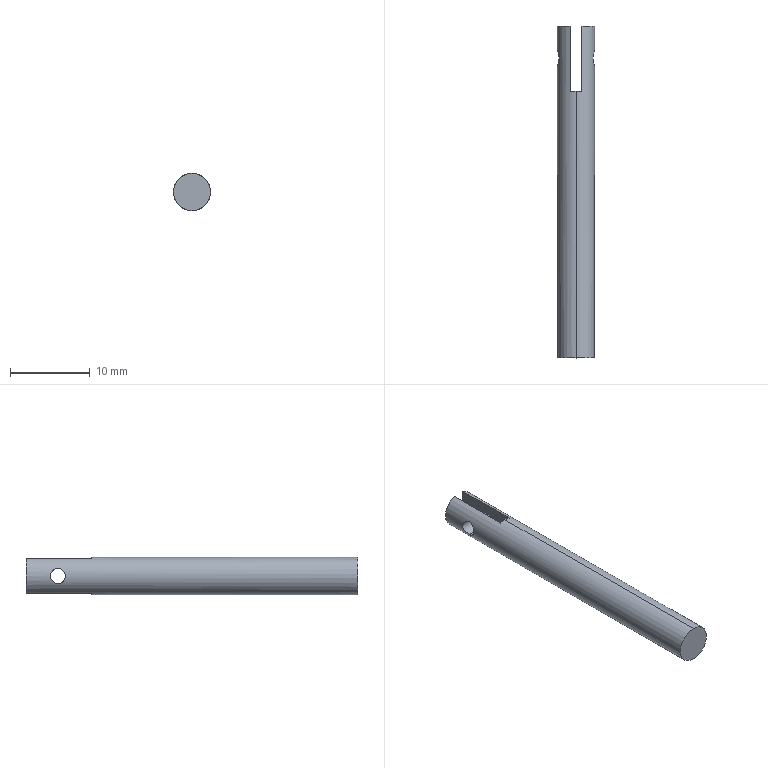Part | SolidWorks | features BaseBody 1 | 1 solid | 12 faces | box 4.65 x 41.6 x 4.65 mm | volume 641.626 mm3 | cylinder 6 | plane 6 | commonest cylinder face diameters 1.9 x4 4.65 x2
STEP:
#1=CARTESIAN_POINT('',(2.122,37.6,-0.95));
#2=VERTEX_POINT('',#1);
#3=CARTESIAN_POINT('',(2.122,37.6,0.95));
#4=VERTEX_POINT('',#3);
#5=CARTESIAN_POINT('',(2.122,37.6,-0.95));
#6=CARTESIAN_POINT('',(2.122,37.473,-0.95));
#7=CARTESIAN_POINT('',(2.134,37.349,-0.9245));
#8=CARTESIAN_POINT('',(2.173,37.119,-0.8288));
#9=CARTESIAN_POINT('',(2.2,37.015,-0.7585));
#10=CARTESIAN_POINT('',(2.252,36.842,-0.5854));
#11=CARTESIAN_POINT('',(2.278,36.771,-0.4807));
#12=CARTESIAN_POINT('',(2.314,36.676,-0.2526));
#13=CARTESIAN_POINT('',(2.325,36.65,-0.1267));
#14=CARTESIAN_POINT('',(2.325,36.65,0.1243));
#15=CARTESIAN_POINT('',(2.315,36.675,0.2495));
#16=CARTESIAN_POINT('',(2.278,36.771,0.4812));
#17=CARTESIAN_POINT('',(2.252,36.841,0.5848));
#18=CARTESIAN_POINT('',(2.2,37.015,0.7586));
#19=CARTESIAN_POINT('',(2.173,37.12,0.8288));
#20=CARTESIAN_POINT('',(2.134,37.347,0.9241));
#21=CARTESIAN_POINT('',(2.122,37.473,0.95));
#22=CARTESIAN_POINT('',(2.122,37.6,0.95));
#23=B_SPLINE_CURVE_WITH_KNOTS('',3,(#5,#6,#7,#8,#9,#10,#11,#12,#13,#14,#15,#16,#17,#18,#19,#20,#21,#22),.UNSPECIFIED.,.F.,.F.,(4,2,2,2,2,2,2,2,4),(0.,0.0003752,0.0007505,0.001126,0.001501,0.001876,0.002251,0.002627,0.003002),.UNSPECIFIED.);
#24=EDGE_CURVE('',#2,#4,#23,.T.);
#25=ORIENTED_EDGE('',*,*,#24,.T.);
#26=CARTESIAN_POINT('',(2.122,37.6,0.95));
#27=CARTESIAN_POINT('',(2.122,37.727,0.95));
#28=CARTESIAN_POINT('',(2.134,37.851,0.9245));
#29=CARTESIAN_POINT('',(2.173,38.081,0.8288));
#30=CARTESIAN_POINT('',(2.2,38.185,0.7585));
#31=CARTESIAN_POINT('',(2.252,38.358,0.5854));
#32=CARTESIAN_POINT('',(2.278,38.429,0.4807));
#33=CARTESIAN_POINT('',(2.314,38.524,0.2526));
#34=CARTESIAN_POINT('',(2.325,38.55,0.1267));
#35=CARTESIAN_POINT('',(2.325,38.55,-0.1243));
#36=CARTESIAN_POINT('',(2.315,38.525,-0.2495));
#37=CARTESIAN_POINT('',(2.278,38.429,-0.4812));
#38=CARTESIAN_POINT('',(2.252,38.359,-0.5848));
#39=CARTESIAN_POINT('',(2.2,38.185,-0.7586));
#40=CARTESIAN_POINT('',(2.173,38.08,-0.8288));
#41=CARTESIAN_POINT('',(2.134,37.853,-0.9241));
#42=CARTESIAN_POINT('',(2.122,37.727,-0.95));
#43=CARTESIAN_POINT('',(2.122,37.6,-0.95));
#44=B_SPLINE_CURVE_WITH_KNOTS('',3,(#26,#27,#28,#29,#30,#31,#32,#33,#34,#35,#36,#37,#38,#39,#40,#41,#42,#43),.UNSPECIFIED.,.F.,.F.,(4,2,2,2,2,2,2,2,4),(0.003002,0.003377,0.003752,0.004127,0.004502,0.004877,0.005253,0.005628,0.006003),.UNSPECIFIED.);
#45=EDGE_CURVE('',#4,#2,#44,.T.);
#46=ORIENTED_EDGE('',*,*,#45,.T.);
#47=EDGE_LOOP('',(#25,#46));
#48=FACE_BOUND('',#47,.T.);
#49=CARTESIAN_POINT('',(0.75,33.4,2.201));
#50=VERTEX_POINT('',#49);
#51=CARTESIAN_POINT('',(0.,33.4,2.325));
#52=VERTEX_POINT('',#51);
#53=CARTESIAN_POINT('',(0.,33.4,0.));
#54=DIRECTION('',(0.,-1.,0.));
#55=DIRECTION('',(0.,0.,-1.));
#56=AXIS2_PLACEMENT_3D('',#53,#54,#55);
#57=CIRCLE('',#56,2.325);
#58=EDGE_CURVE('',#50,#52,#57,.T.);
#59=ORIENTED_EDGE('',*,*,#58,.T.);
#60=CARTESIAN_POINT('',(0.,0.,2.325));
#61=VERTEX_POINT('',#60);
#62=CARTESIAN_POINT('',(0.,41.6,2.325));
#63=DIRECTION('',(0.,-1.,0.));
#64=VECTOR('',#63,1000.);
#65=LINE('',#62,#64);
#66=EDGE_CURVE('',#52,#61,#65,.T.);
#67=ORIENTED_EDGE('',*,*,#66,.T.);
#68=CARTESIAN_POINT('',(0.,0.,-2.325));
#69=VERTEX_POINT('',#68);
#70=CARTESIAN_POINT('',(0.,0.,0.));
#71=DIRECTION('',(0.,1.,0.));
#72=DIRECTION('',(0.,0.,-1.));
#73=AXIS2_PLACEMENT_3D('',#70,#71,#72);
#74=CIRCLE('',#73,2.325);
#75=EDGE_CURVE('',#61,#69,#74,.T.);
#76=ORIENTED_EDGE('',*,*,#75,.T.);
#77=CARTESIAN_POINT('',(0.,33.4,-2.325));
#78=VERTEX_POINT('',#77);
#79=CARTESIAN_POINT('',(0.,41.6,-2.325));
#80=DIRECTION('',(0.,-1.,0.));
#81=VECTOR('',#80,1000.);
#82=LINE('',#79,#81);
#83=EDGE_CURVE('',#78,#69,#82,.T.);
#84=ORIENTED_EDGE('',*,*,#83,.F.);
#85=CARTESIAN_POINT('',(0.75,33.4,-2.201));
#86=VERTEX_POINT('',#85);
#87=CARTESIAN_POINT('',(0.,33.4,0.));
#88=DIRECTION('',(0.,-1.,0.));
#89=DIRECTION('',(0.,0.,-1.));
#90=AXIS2_PLACEMENT_3D('',#87,#88,#89);
#91=CIRCLE('',#90,2.325);
#92=EDGE_CURVE('',#78,#86,#91,.T.);
#93=ORIENTED_EDGE('',*,*,#92,.T.);
#94=CARTESIAN_POINT('',(0.75,41.6,-2.201));
#95=VERTEX_POINT('',#94);
#96=CARTESIAN_POINT('',(0.75,41.6,-2.201));
#97=DIRECTION('',(0.,1.,0.));
#98=VECTOR('',#97,1000.);
#99=LINE('',#96,#98);
#100=EDGE_CURVE('',#86,#95,#99,.T.);
#101=ORIENTED_EDGE('',*,*,#100,.T.);
#102=CARTESIAN_POINT('',(0.75,41.6,2.201));
#103=VERTEX_POINT('',#102);
#104=CARTESIAN_POINT('',(0.,41.6,0.));
#105=DIRECTION('',(0.,-1.,0.));
#106=DIRECTION('',(0.,0.,-1.));
#107=AXIS2_PLACEMENT_3D('',#104,#105,#106);
#108=CIRCLE('',#107,2.325);
#109=EDGE_CURVE('',#95,#103,#108,.T.);
#110=ORIENTED_EDGE('',*,*,#109,.T.);
#111=CARTESIAN_POINT('',(0.75,41.6,2.201));
#112=DIRECTION('',(0.,-1.,0.));
#113=VECTOR('',#112,1000.);
#114=LINE('',#111,#113);
#115=EDGE_CURVE('',#103,#50,#114,.T.);
#116=ORIENTED_EDGE('',*,*,#115,.T.);
#117=EDGE_LOOP('',(#59,#67,#76,#84,#93,#101,#110,#116));
#118=FACE_OUTER_BOUND('',#117,.T.);
#119=CARTESIAN_POINT('',(0.,41.6,0.));
#120=DIRECTION('',(0.,-1.,0.));
#121=DIRECTION('',(0.,0.,-1.));
#122=AXIS2_PLACEMENT_3D('',#119,#120,#121);
#123=CYLINDRICAL_SURFACE('',#122,2.325);
#124=ADVANCED_FACE('',(#48,#118),#123,.T.);
#125=CARTESIAN_POINT('',(0.75,37.6,-0.95));
#126=VERTEX_POINT('',#125);
#127=CARTESIAN_POINT('',(0.75,37.6,0.95));
#128=VERTEX_POINT('',#127);
#129=CARTESIAN_POINT('',(0.75,37.6,0.));
#130=DIRECTION('',(-1.,0.,0.));
#131=DIRECTION('',(0.,0.,-1.));
#132=AXIS2_PLACEMENT_3D('',#129,#130,#131);
#133=CIRCLE('',#132,0.95);
#134=EDGE_CURVE('',#126,#128,#133,.T.);
#135=ORIENTED_EDGE('',*,*,#134,.T.);
#136=CARTESIAN_POINT('',(-4.85,37.6,0.95));
#137=DIRECTION('',(1.,0.,0.));
#138=VECTOR('',#137,1000.);
#139=LINE('',#136,#138);
#140=EDGE_CURVE('',#128,#4,#139,.T.);
#141=ORIENTED_EDGE('',*,*,#140,.T.);
#142=ORIENTED_EDGE('',*,*,#24,.F.);
#143=CARTESIAN_POINT('',(-4.85,37.6,-0.95));
#144=DIRECTION('',(1.,0.,0.));
#145=VECTOR('',#144,1000.);
#146=LINE('',#143,#145);
#147=EDGE_CURVE('',#126,#2,#146,.T.);
#148=ORIENTED_EDGE('',*,*,#147,.F.);
#149=EDGE_LOOP('',(#135,#141,#142,#148));
#150=FACE_OUTER_BOUND('',#149,.T.);
#151=CARTESIAN_POINT('',(-4.85,37.6,0.));
#152=DIRECTION('',(1.,0.,0.));
#153=DIRECTION('',(0.,0.,-1.));
#154=AXIS2_PLACEMENT_3D('',#151,#152,#153);
#155=CYLINDRICAL_SURFACE('',#154,0.95);
#156=ADVANCED_FACE('',(#150),#155,.F.);
#157=CARTESIAN_POINT('',(-2.122,37.6,0.95));
#158=VERTEX_POINT('',#157);
#159=CARTESIAN_POINT('',(-2.122,37.6,-0.95));
#160=VERTEX_POINT('',#159);
#161=CARTESIAN_POINT('',(-2.122,37.6,0.95));
#162=CARTESIAN_POINT('',(-2.122,37.473,0.95));
#163=CARTESIAN_POINT('',(-2.134,37.349,0.9245));
#164=CARTESIAN_POINT('',(-2.173,37.119,0.8288));
#165=CARTESIAN_POINT('',(-2.2,37.015,0.7585));
#166=CARTESIAN_POINT('',(-2.252,36.842,0.5854));
#167=CARTESIAN_POINT('',(-2.278,36.771,0.4807));
#168=CARTESIAN_POINT('',(-2.314,36.676,0.2526));
#169=CARTESIAN_POINT('',(-2.325,36.65,0.1267));
#170=CARTESIAN_POINT('',(-2.325,36.65,-0.1243));
#171=CARTESIAN_POINT('',(-2.315,36.675,-0.2495));
#172=CARTESIAN_POINT('',(-2.278,36.771,-0.4812));
#173=CARTESIAN_POINT('',(-2.252,36.841,-0.5848));
#174=CARTESIAN_POINT('',(-2.2,37.015,-0.7586));
#175=CARTESIAN_POINT('',(-2.173,37.12,-0.8288));
#176=CARTESIAN_POINT('',(-2.134,37.347,-0.9241));
#177=CARTESIAN_POINT('',(-2.122,37.473,-0.95));
#178=CARTESIAN_POINT('',(-2.122,37.6,-0.95));
#179=B_SPLINE_CURVE_WITH_KNOTS('',3,(#161,#162,#163,#164,#165,#166,#167,#168,#169,#170,#171,#172,#173,#174,#175,#176,#177,#178),.UNSPECIFIED.,.F.,.F.,(4,2,2,2,2,2,2,2,4),(0.,0.0003752,0.0007505,0.001126,0.001501,0.001876,0.002251,0.002627,0.003002),.UNSPECIFIED.);
#180=EDGE_CURVE('',#158,#160,#179,.T.);
#181=ORIENTED_EDGE('',*,*,#180,.F.);
#182=CARTESIAN_POINT('',(-0.75,37.6,0.95));
#183=VERTEX_POINT('',#182);
#184=CARTESIAN_POINT('',(-4.85,37.6,0.95));
#185=DIRECTION('',(1.,0.,0.));
#186=VECTOR('',#185,1000.);
#187=LINE('',#184,#186);
#188=EDGE_CURVE('',#158,#183,#187,.T.);
#189=ORIENTED_EDGE('',*,*,#188,.T.);
#190=CARTESIAN_POINT('',(-0.75,37.6,-0.95));
#191=VERTEX_POINT('',#190);
#192=CARTESIAN_POINT('',(-0.75,37.6,0.));
#193=DIRECTION('',(-1.,0.,0.));
#194=DIRECTION('',(0.,0.,-1.));
#195=AXIS2_PLACEMENT_3D('',#192,#193,#194);
#196=CIRCLE('',#195,0.95);
#197=EDGE_CURVE('',#191,#183,#196,.T.);
#198=ORIENTED_EDGE('',*,*,#197,.F.);
#199=CARTESIAN_POINT('',(-4.85,37.6,-0.95));
#200=DIRECTION('',(1.,0.,0.));
#201=VECTOR('',#200,1000.);
#202=LINE('',#199,#201);
#203=EDGE_CURVE('',#160,#191,#202,.T.);
#204=ORIENTED_EDGE('',*,*,#203,.F.);
#205=EDGE_LOOP('',(#181,#189,#198,#204));
#206=FACE_OUTER_BOUND('',#205,.T.);
#207=CARTESIAN_POINT('',(-4.85,37.6,0.));
#208=DIRECTION('',(1.,0.,0.));
#209=DIRECTION('',(0.,0.,-1.));
#210=AXIS2_PLACEMENT_3D('',#207,#208,#209);
#211=CYLINDRICAL_SURFACE('',#210,0.95);
#212=ADVANCED_FACE('',(#206),#211,.F.);
#213=ORIENTED_EDGE('',*,*,#66,.F.);
#214=CARTESIAN_POINT('',(-0.75,33.4,2.201));
#215=VERTEX_POINT('',#214);
#216=CARTESIAN_POINT('',(0.,33.4,0.));
#217=DIRECTION('',(0.,-1.,0.));
#218=DIRECTION('',(0.,0.,-1.));
#219=AXIS2_PLACEMENT_3D('',#216,#217,#218);
#220=CIRCLE('',#219,2.325);
#221=EDGE_CURVE('',#52,#215,#220,.T.);
#222=ORIENTED_EDGE('',*,*,#221,.T.);
#223=CARTESIAN_POINT('',(-0.75,41.6,2.201));
#224=VERTEX_POINT('',#223);
#225=CARTESIAN_POINT('',(-0.75,41.6,2.201));
#226=DIRECTION('',(0.,1.,0.));
#227=VECTOR('',#226,1000.);
#228=LINE('',#225,#227);
#229=EDGE_CURVE('',#215,#224,#228,.T.);
#230=ORIENTED_EDGE('',*,*,#229,.T.);
#231=CARTESIAN_POINT('',(-0.75,41.6,-2.201));
#232=VERTEX_POINT('',#231);
#233=CARTESIAN_POINT('',(0.,41.6,0.));
#234=DIRECTION('',(0.,-1.,0.));
#235=DIRECTION('',(0.,0.,-1.));
#236=AXIS2_PLACEMENT_3D('',#233,#234,#235);
#237=CIRCLE('',#236,2.325);
#238=EDGE_CURVE('',#224,#232,#237,.T.);
#239=ORIENTED_EDGE('',*,*,#238,.T.);
#240=CARTESIAN_POINT('',(-0.75,33.4,-2.201));
#241=VERTEX_POINT('',#240);
#242=CARTESIAN_POINT('',(-0.75,41.6,-2.201));
#243=DIRECTION('',(0.,-1.,0.));
#244=VECTOR('',#243,1000.);
#245=LINE('',#242,#244);
#246=EDGE_CURVE('',#232,#241,#245,.T.);
#247=ORIENTED_EDGE('',*,*,#246,.T.);
#248=CARTESIAN_POINT('',(0.,33.4,0.));
#249=DIRECTION('',(0.,-1.,0.));
#250=DIRECTION('',(0.,0.,-1.));
#251=AXIS2_PLACEMENT_3D('',#248,#249,#250);
#252=CIRCLE('',#251,2.325);
#253=EDGE_CURVE('',#241,#78,#252,.T.);
#254=ORIENTED_EDGE('',*,*,#253,.T.);
#255=ORIENTED_EDGE('',*,*,#83,.T.);
#256=CARTESIAN_POINT('',(0.,0.,0.));
#257=DIRECTION('',(0.,1.,0.));
#258=DIRECTION('',(0.,0.,-1.));
#259=AXIS2_PLACEMENT_3D('',#256,#257,#258);
#260=CIRCLE('',#259,2.325);
#261=EDGE_CURVE('',#69,#61,#260,.T.);
#262=ORIENTED_EDGE('',*,*,#261,.T.);
#263=EDGE_LOOP('',(#213,#222,#230,#239,#247,#254,#255,#262));
#264=FACE_OUTER_BOUND('',#263,.T.);
#265=CARTESIAN_POINT('',(-2.122,37.6,-0.95));
#266=CARTESIAN_POINT('',(-2.122,37.727,-0.95));
#267=CARTESIAN_POINT('',(-2.134,37.851,-0.9245));
#268=CARTESIAN_POINT('',(-2.173,38.081,-0.8288));
#269=CARTESIAN_POINT('',(-2.2,38.185,-0.7585));
#270=CARTESIAN_POINT('',(-2.252,38.358,-0.5854));
#271=CARTESIAN_POINT('',(-2.278,38.429,-0.4807));
#272=CARTESIAN_POINT('',(-2.314,38.524,-0.2526));
#273=CARTESIAN_POINT('',(-2.325,38.55,-0.1267));
#274=CARTESIAN_POINT('',(-2.325,38.55,0.1243));
#275=CARTESIAN_POINT('',(-2.315,38.525,0.2495));
#276=CARTESIAN_POINT('',(-2.278,38.429,0.4812));
#277=CARTESIAN_POINT('',(-2.252,38.359,0.5848));
#278=CARTESIAN_POINT('',(-2.2,38.185,0.7586));
#279=CARTESIAN_POINT('',(-2.173,38.08,0.8288));
#280=CARTESIAN_POINT('',(-2.134,37.853,0.9241));
#281=CARTESIAN_POINT('',(-2.122,37.727,0.95));
#282=CARTESIAN_POINT('',(-2.122,37.6,0.95));
#283=B_SPLINE_CURVE_WITH_KNOTS('',3,(#265,#266,#267,#268,#269,#270,#271,#272,#273,#274,#275,#276,#277,#278,#279,#280,#281,#282),.UNSPECIFIED.,.F.,.F.,(4,2,2,2,2,2,2,2,4),(0.003002,0.003377,0.003752,0.004127,0.004502,0.004877,0.005253,0.005628,0.006003),.UNSPECIFIED.);
#284=EDGE_CURVE('',#160,#158,#283,.T.);
#285=ORIENTED_EDGE('',*,*,#284,.T.);
#286=ORIENTED_EDGE('',*,*,#180,.T.);
#287=EDGE_LOOP('',(#285,#286));
#288=FACE_BOUND('',#287,.T.);
#289=CARTESIAN_POINT('',(0.,41.6,0.));
#290=DIRECTION('',(0.,-1.,0.));
#291=DIRECTION('',(0.,0.,-1.));
#292=AXIS2_PLACEMENT_3D('',#289,#290,#291);
#293=CYLINDRICAL_SURFACE('',#292,2.325);
#294=ADVANCED_FACE('',(#264,#288),#293,.T.);
#295=ORIENTED_EDGE('',*,*,#134,.F.);
#296=CARTESIAN_POINT('',(0.75,37.6,0.));
#297=DIRECTION('',(-1.,0.,0.));
#298=DIRECTION('',(0.,0.,-1.));
#299=AXIS2_PLACEMENT_3D('',#296,#297,#298);
#300=CIRCLE('',#299,0.95);
#301=EDGE_CURVE('',#128,#126,#300,.T.);
#302=ORIENTED_EDGE('',*,*,#301,.F.);
#303=EDGE_LOOP('',(#295,#302));
#304=FACE_BOUND('',#303,.T.);
#305=CARTESIAN_POINT('',(0.75,33.4,-4.96));
#306=DIRECTION('',(0.,0.,-1.));
#307=VECTOR('',#306,1000.);
#308=LINE('',#305,#307);
#309=EDGE_CURVE('',#50,#86,#308,.T.);
#310=ORIENTED_EDGE('',*,*,#309,.F.);
#311=ORIENTED_EDGE('',*,*,#115,.F.);
#312=CARTESIAN_POINT('',(0.75,41.6,-4.96));
#313=DIRECTION('',(0.,0.,1.));
#314=VECTOR('',#313,1000.);
#315=LINE('',#312,#314);
#316=EDGE_CURVE('',#95,#103,#315,.T.);
#317=ORIENTED_EDGE('',*,*,#316,.F.);
#318=ORIENTED_EDGE('',*,*,#100,.F.);
#319=EDGE_LOOP('',(#310,#311,#317,#318));
#320=FACE_OUTER_BOUND('',#319,.T.);
#321=CARTESIAN_POINT('',(0.75,33.4,-4.96));
#322=DIRECTION('',(1.,0.,0.));
#323=DIRECTION('',(0.,0.,-1.));
#324=AXIS2_PLACEMENT_3D('',#321,#322,#323);
#325=PLANE('',#324);
#326=ADVANCED_FACE('',(#304,#320),#325,.F.);
#327=ORIENTED_EDGE('',*,*,#316,.T.);
#328=ORIENTED_EDGE('',*,*,#109,.F.);
#329=EDGE_LOOP('',(#327,#328));
#330=FACE_OUTER_BOUND('',#329,.T.);
#331=CARTESIAN_POINT('',(0.,41.6,0.));
#332=DIRECTION('',(0.,1.,0.));
#333=DIRECTION('',(0.,0.,1.));
#334=AXIS2_PLACEMENT_3D('',#331,#332,#333);
#335=PLANE('',#334);
#336=ADVANCED_FACE('',(#330),#335,.T.);
#337=ORIENTED_EDGE('',*,*,#261,.F.);
#338=ORIENTED_EDGE('',*,*,#75,.F.);
#339=EDGE_LOOP('',(#337,#338));
#340=FACE_OUTER_BOUND('',#339,.T.);
#341=CARTESIAN_POINT('',(0.,0.,0.));
#342=DIRECTION('',(0.,1.,0.));
#343=DIRECTION('',(0.,0.,1.));
#344=AXIS2_PLACEMENT_3D('',#341,#342,#343);
#345=PLANE('',#344);
#346=ADVANCED_FACE('',(#340),#345,.F.);
#347=ORIENTED_EDGE('',*,*,#140,.F.);
#348=ORIENTED_EDGE('',*,*,#301,.T.);
#349=ORIENTED_EDGE('',*,*,#147,.T.);
#350=ORIENTED_EDGE('',*,*,#45,.F.);
#351=EDGE_LOOP('',(#347,#348,#349,#350));
#352=FACE_OUTER_BOUND('',#351,.T.);
#353=CARTESIAN_POINT('',(-4.85,37.6,0.));
#354=DIRECTION('',(1.,0.,0.));
#355=DIRECTION('',(0.,0.,-1.));
#356=AXIS2_PLACEMENT_3D('',#353,#354,#355);
#357=CYLINDRICAL_SURFACE('',#356,0.95);
#358=ADVANCED_FACE('',(#352),#357,.F.);
#359=ORIENTED_EDGE('',*,*,#309,.T.);
#360=ORIENTED_EDGE('',*,*,#92,.F.);
#361=ORIENTED_EDGE('',*,*,#253,.F.);
#362=CARTESIAN_POINT('',(-0.75,33.4,0.));
#363=DIRECTION('',(0.,0.,-1.));
#364=VECTOR('',#363,1000.);
#365=LINE('',#362,#364);
#366=EDGE_CURVE('',#215,#241,#365,.T.);
#367=ORIENTED_EDGE('',*,*,#366,.F.);
#368=ORIENTED_EDGE('',*,*,#221,.F.);
#369=ORIENTED_EDGE('',*,*,#58,.F.);
#370=EDGE_LOOP('',(#359,#360,#361,#367,#368,#369));
#371=FACE_OUTER_BOUND('',#370,.T.);
#372=CARTESIAN_POINT('',(0.,33.4,0.));
#373=DIRECTION('',(0.,-1.,0.));
#374=DIRECTION('',(0.,0.,-1.));
#375=AXIS2_PLACEMENT_3D('',#372,#373,#374);
#376=PLANE('',#375);
#377=ADVANCED_FACE('',(#371),#376,.F.);
#378=ORIENTED_EDGE('',*,*,#188,.F.);
#379=ORIENTED_EDGE('',*,*,#284,.F.);
#380=ORIENTED_EDGE('',*,*,#203,.T.);
#381=CARTESIAN_POINT('',(-0.75,37.6,0.));
#382=DIRECTION('',(-1.,0.,0.));
#383=DIRECTION('',(0.,0.,-1.));
#384=AXIS2_PLACEMENT_3D('',#381,#382,#383);
#385=CIRCLE('',#384,0.95);
#386=EDGE_CURVE('',#183,#191,#385,.T.);
#387=ORIENTED_EDGE('',*,*,#386,.F.);
#388=EDGE_LOOP('',(#378,#379,#380,#387));
#389=FACE_OUTER_BOUND('',#388,.T.);
#390=CARTESIAN_POINT('',(-4.85,37.6,0.));
#391=DIRECTION('',(1.,0.,0.));
#392=DIRECTION('',(0.,0.,-1.));
#393=AXIS2_PLACEMENT_3D('',#390,#391,#392);
#394=CYLINDRICAL_SURFACE('',#393,0.95);
#395=ADVANCED_FACE('',(#389),#394,.F.);
#396=ORIENTED_EDGE('',*,*,#197,.T.);
#397=ORIENTED_EDGE('',*,*,#386,.T.);
#398=EDGE_LOOP('',(#396,#397));
#399=FACE_BOUND('',#398,.T.);
#400=ORIENTED_EDGE('',*,*,#366,.T.);
#401=ORIENTED_EDGE('',*,*,#246,.F.);
#402=CARTESIAN_POINT('',(-0.75,41.6,0.));
#403=DIRECTION('',(0.,0.,-1.));
#404=VECTOR('',#403,1000.);
#405=LINE('',#402,#404);
#406=EDGE_CURVE('',#224,#232,#405,.T.);
#407=ORIENTED_EDGE('',*,*,#406,.F.);
#408=ORIENTED_EDGE('',*,*,#229,.F.);
#409=EDGE_LOOP('',(#400,#401,#407,#408));
#410=FACE_OUTER_BOUND('',#409,.T.);
#411=CARTESIAN_POINT('',(-0.75,33.4,0.));
#412=DIRECTION('',(-1.,0.,0.));
#413=DIRECTION('',(0.,0.,1.));
#414=AXIS2_PLACEMENT_3D('',#411,#412,#413);
#415=PLANE('',#414);
#416=ADVANCED_FACE('',(#399,#410),#415,.F.);
#417=ORIENTED_EDGE('',*,*,#406,.T.);
#418=ORIENTED_EDGE('',*,*,#238,.F.);
#419=EDGE_LOOP('',(#417,#418));
#420=FACE_OUTER_BOUND('',#419,.T.);
#421=CARTESIAN_POINT('',(0.,41.6,0.));
#422=DIRECTION('',(0.,1.,0.));
#423=DIRECTION('',(0.,0.,1.));
#424=AXIS2_PLACEMENT_3D('',#421,#422,#423);
#425=PLANE('',#424);
#426=ADVANCED_FACE('',(#420),#425,.T.);
#427=CLOSED_SHELL('',(#124,#156,#212,#294,#326,#336,#346,#358,#377,#395,#416,#426));
#428=MANIFOLD_SOLID_BREP('',#427);
#429=CARTESIAN_POINT('',(0.,0.,0.));
#430=DIRECTION('',(0.,0.,1.));
#431=DIRECTION('',(1.,0.,0.));
#432=AXIS2_PLACEMENT_3D('',#429,#430,#431);
#433=(LENGTH_UNIT()NAMED_UNIT(*)SI_UNIT(.MILLI.,.METRE.));
#434=UNCERTAINTY_MEASURE_WITH_UNIT(LENGTH_MEASURE(0.00001),#433,'','');
#435=(NAMED_UNIT(*)PLANE_ANGLE_UNIT()SI_UNIT($,.RADIAN.));
#436=(NAMED_UNIT(*)SI_UNIT($,.STERADIAN.)SOLID_ANGLE_UNIT());
#437=(GEOMETRIC_REPRESENTATION_CONTEXT(3)GLOBAL_UNCERTAINTY_ASSIGNED_CONTEXT((#434))GLOBAL_UNIT_ASSIGNED_CONTEXT((#433,#435,#436))REPRESENTATION_CONTEXT('',''));
#438=ADVANCED_BREP_SHAPE_REPRESENTATION('',(#428,#432),#437);